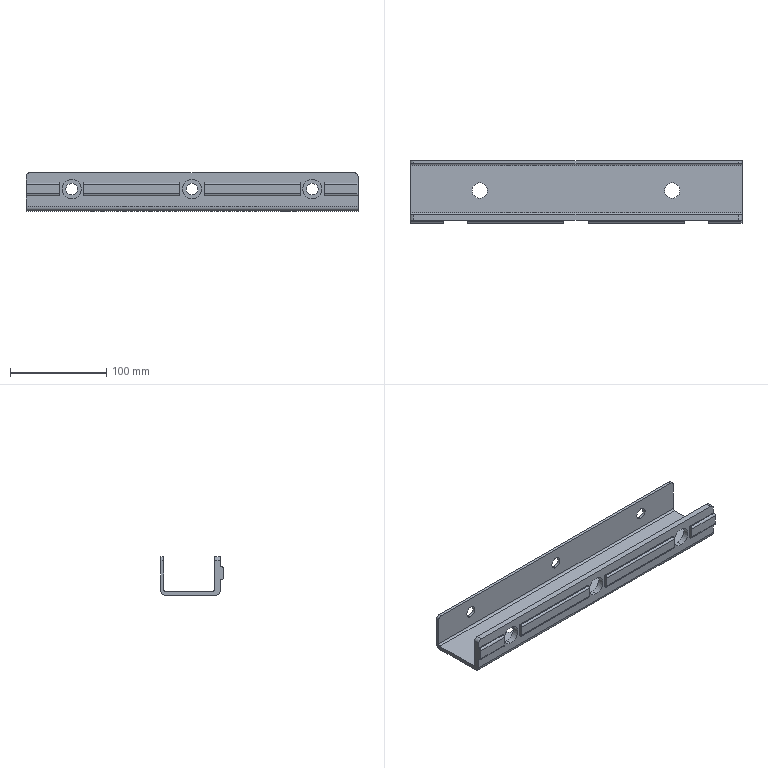Part | STEP file | Screen clamp | 1 solid | 60 faces | box 345 x 65 x 40 mm | volume 196764 mm3 | cylinder 32 | plane 28 | commonest cylinder face diameters 4 x10 12 x6 20 x6 8 x4 16 x4 10 x2